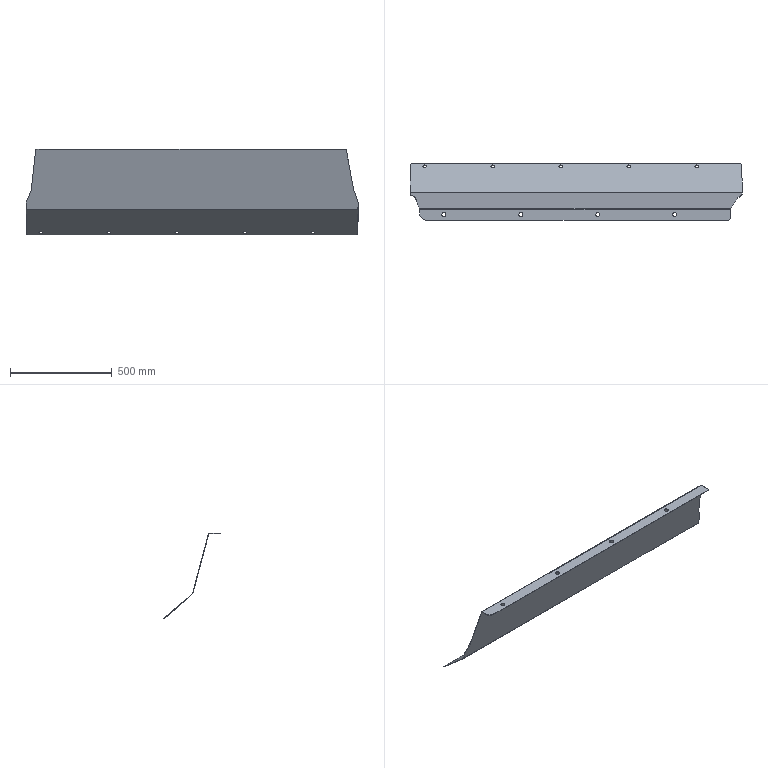Part | SolidWorks | features SM3dBend 2, FlatPattern 1, SMBaseFlange 1, SheetMetal 1 | 1 solid | 54 faces | box 1635 x 277.618 x 421.117 mm | volume 1397928 mm3 | cylinder 30 | plane 22 | spline 2 | commonest cylinder face diameters 20 x11 18 x10 100 x4 3 x2 6.2 x2 60 x1